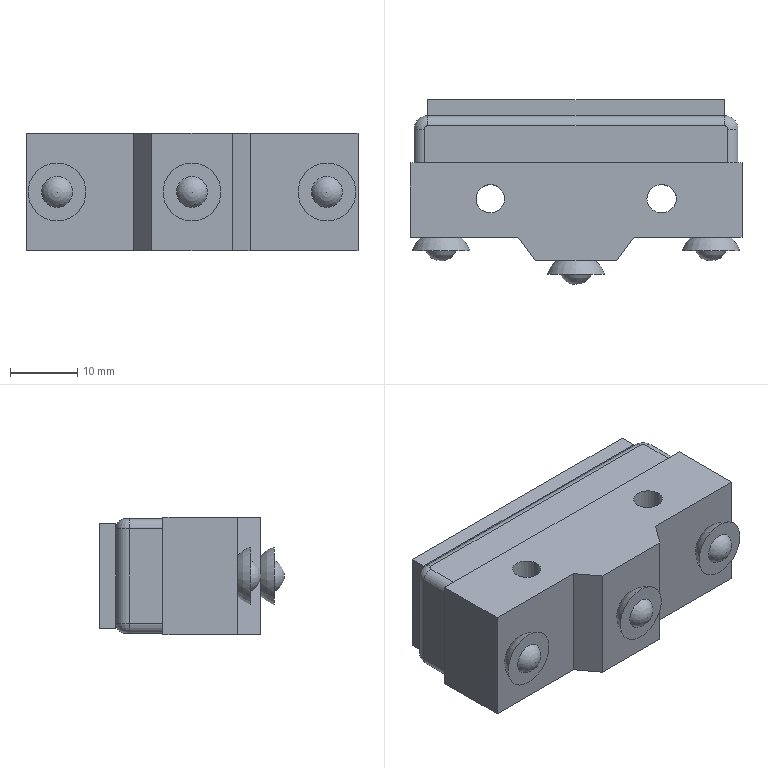Part | NX | features MFD10-WL40_1 2 | 1 solid | 44 faces | box 49.2 x 27.4 x 17.45 mm | volume 17430 mm3 | plane 24 | cylinder 9 | sphere 6 | torus 4 | spline 1 | commonest cylinder face diameters 3 x6 4 x2 4.2 x1
STEP:
#1=CARTESIAN_POINT('',(255.829,-488.15,79.));
#2=VERTEX_POINT('',#1);
#3=CARTESIAN_POINT('',(239.829,-488.15,79.));
#4=VERTEX_POINT('',#3);
#5=CARTESIAN_POINT('',(255.829,-488.15,79.));
#6=DIRECTION('',(-1.,0.,0.));
#7=VECTOR('',#6,1000.);
#8=LINE('',#5,#7);
#9=EDGE_CURVE('',#2,#4,#8,.T.);
#10=ORIENTED_EDGE('',*,*,#9,.F.);
#11=CARTESIAN_POINT('',(255.829,-488.15,96.45));
#12=VERTEX_POINT('',#11);
#13=CARTESIAN_POINT('',(255.829,-488.15,96.45));
#14=DIRECTION('',(0.,0.,-1.));
#15=VECTOR('',#14,1000.);
#16=LINE('',#13,#15);
#17=EDGE_CURVE('',#12,#2,#16,.T.);
#18=ORIENTED_EDGE('',*,*,#17,.F.);
#19=CARTESIAN_POINT('',(239.829,-488.15,96.45));
#20=VERTEX_POINT('',#19);
#21=CARTESIAN_POINT('',(255.829,-488.15,96.45));
#22=DIRECTION('',(-1.,0.,0.));
#23=VECTOR('',#22,1000.);
#24=LINE('',#21,#23);
#25=EDGE_CURVE('',#12,#20,#24,.T.);
#26=ORIENTED_EDGE('',*,*,#25,.T.);
#27=CARTESIAN_POINT('',(239.829,-488.15,96.45));
#28=DIRECTION('',(0.,0.,-1.));
#29=VECTOR('',#28,1000.);
#30=LINE('',#27,#29);
#31=EDGE_CURVE('',#20,#4,#30,.T.);
#32=ORIENTED_EDGE('',*,*,#31,.T.);
#33=EDGE_LOOP('',(#10,#18,#26,#32));
#34=FACE_BOUND('',#33,.T.);
#35=CARTESIAN_POINT('',(244.429,-488.15,90.725));
#36=VERTEX_POINT('',#35);
#37=CARTESIAN_POINT('',(244.429,-488.15,87.725));
#38=DIRECTION('',(0.,1.,0.));
#39=DIRECTION('',(0.,0.,1.));
#40=AXIS2_PLACEMENT_3D('',#37,#38,#39);
#41=CIRCLE('',#40,3.);
#42=EDGE_CURVE('',#36,#36,#41,.T.);
#43=ORIENTED_EDGE('',*,*,#42,.T.);
#44=EDGE_LOOP('',(#43));
#45=FACE_BOUND('',#44,.T.);
#46=CARTESIAN_POINT('',(255.829,-488.15,96.45));
#47=DIRECTION('',(0.,-1.,0.));
#48=DIRECTION('',(0.,0.,1.));
#49=AXIS2_PLACEMENT_3D('',#46,#47,#48);
#50=PLANE('',#49);
#51=ADVANCED_FACE('',(#34,#45),#50,.T.);
#52=CARTESIAN_POINT('',(289.029,-488.15,79.));
#53=VERTEX_POINT('',#52);
#54=CARTESIAN_POINT('',(273.029,-488.15,79.));
#55=VERTEX_POINT('',#54);
#56=CARTESIAN_POINT('',(289.029,-488.15,79.));
#57=DIRECTION('',(-1.,0.,0.));
#58=VECTOR('',#57,1000.);
#59=LINE('',#56,#58);
#60=EDGE_CURVE('',#53,#55,#59,.T.);
#61=ORIENTED_EDGE('',*,*,#60,.F.);
#62=CARTESIAN_POINT('',(289.029,-488.15,96.45));
#63=VERTEX_POINT('',#62);
#64=CARTESIAN_POINT('',(289.029,-488.15,96.45));
#65=DIRECTION('',(0.,0.,-1.));
#66=VECTOR('',#65,1000.);
#67=LINE('',#64,#66);
#68=EDGE_CURVE('',#63,#53,#67,.T.);
#69=ORIENTED_EDGE('',*,*,#68,.F.);
#70=CARTESIAN_POINT('',(273.029,-488.15,96.45));
#71=VERTEX_POINT('',#70);
#72=CARTESIAN_POINT('',(289.029,-488.15,96.45));
#73=DIRECTION('',(-1.,0.,0.));
#74=VECTOR('',#73,1000.);
#75=LINE('',#72,#74);
#76=EDGE_CURVE('',#63,#71,#75,.T.);
#77=ORIENTED_EDGE('',*,*,#76,.T.);
#78=CARTESIAN_POINT('',(273.029,-488.15,96.45));
#79=DIRECTION('',(0.,0.,-1.));
#80=VECTOR('',#79,1000.);
#81=LINE('',#78,#80);
#82=EDGE_CURVE('',#71,#55,#81,.T.);
#83=ORIENTED_EDGE('',*,*,#82,.T.);
#84=EDGE_LOOP('',(#61,#69,#77,#83));
#85=FACE_BOUND('',#84,.T.);
#86=CARTESIAN_POINT('',(284.429,-488.15,90.725));
#87=VERTEX_POINT('',#86);
#88=CARTESIAN_POINT('',(284.429,-488.15,87.725));
#89=DIRECTION('',(0.,-1.,0.));
#90=DIRECTION('',(0.,0.,1.));
#91=AXIS2_PLACEMENT_3D('',#88,#89,#90);
#92=CIRCLE('',#91,3.);
#93=EDGE_CURVE('',#87,#87,#92,.T.);
#94=ORIENTED_EDGE('',*,*,#93,.F.);
#95=EDGE_LOOP('',(#94));
#96=FACE_BOUND('',#95,.T.);
#97=CARTESIAN_POINT('',(289.029,-488.15,96.45));
#98=DIRECTION('',(0.,-1.,0.));
#99=DIRECTION('',(0.,0.,1.));
#100=AXIS2_PLACEMENT_3D('',#97,#98,#99);
#101=PLANE('',#100);
#102=ADVANCED_FACE('',(#85,#96),#101,.T.);
#103=CARTESIAN_POINT('',(270.429,-491.65,79.));
#104=VERTEX_POINT('',#103);
#105=CARTESIAN_POINT('',(258.429,-491.65,79.));
#106=VERTEX_POINT('',#105);
#107=CARTESIAN_POINT('',(270.429,-491.65,79.));
#108=DIRECTION('',(-1.,0.,0.));
#109=VECTOR('',#108,1000.);
#110=LINE('',#107,#109);
#111=EDGE_CURVE('',#104,#106,#110,.T.);
#112=ORIENTED_EDGE('',*,*,#111,.F.);
#113=CARTESIAN_POINT('',(270.429,-491.65,96.45));
#114=VERTEX_POINT('',#113);
#115=CARTESIAN_POINT('',(270.429,-491.65,96.45));
#116=DIRECTION('',(0.,0.,-1.));
#117=VECTOR('',#116,1000.);
#118=LINE('',#115,#117);
#119=EDGE_CURVE('',#114,#104,#118,.T.);
#120=ORIENTED_EDGE('',*,*,#119,.F.);
#121=CARTESIAN_POINT('',(258.429,-491.65,96.45));
#122=VERTEX_POINT('',#121);
#123=CARTESIAN_POINT('',(270.429,-491.65,96.45));
#124=DIRECTION('',(-1.,0.,0.));
#125=VECTOR('',#124,1000.);
#126=LINE('',#123,#125);
#127=EDGE_CURVE('',#114,#122,#126,.T.);
#128=ORIENTED_EDGE('',*,*,#127,.T.);
#129=CARTESIAN_POINT('',(258.429,-491.65,96.45));
#130=DIRECTION('',(0.,0.,-1.));
#131=VECTOR('',#130,1000.);
#132=LINE('',#129,#131);
#133=EDGE_CURVE('',#122,#106,#132,.T.);
#134=ORIENTED_EDGE('',*,*,#133,.T.);
#135=EDGE_LOOP('',(#112,#120,#128,#134));
#136=FACE_BOUND('',#135,.T.);
#137=CARTESIAN_POINT('',(264.429,-491.65,90.725));
#138=VERTEX_POINT('',#137);
#139=CARTESIAN_POINT('',(264.429,-491.65,87.725));
#140=DIRECTION('',(0.,-1.,0.));
#141=DIRECTION('',(0.,0.,1.));
#142=AXIS2_PLACEMENT_3D('',#139,#140,#141);
#143=CIRCLE('',#142,3.);
#144=EDGE_CURVE('',#138,#138,#143,.T.);
#145=ORIENTED_EDGE('',*,*,#144,.F.);
#146=EDGE_LOOP('',(#145));
#147=FACE_BOUND('',#146,.T.);
#148=CARTESIAN_POINT('',(270.429,-491.65,96.45));
#149=DIRECTION('',(0.,-1.,0.));
#150=DIRECTION('',(0.,0.,1.));
#151=AXIS2_PLACEMENT_3D('',#148,#149,#150);
#152=PLANE('',#151);
#153=ADVANCED_FACE('',(#136,#147),#152,.T.);
#154=CARTESIAN_POINT('',(273.029,-488.15,79.));
#155=DIRECTION('',(-0.5963,-0.8027,0.));
#156=VECTOR('',#155,1000.);
#157=LINE('',#154,#156);
#158=EDGE_CURVE('',#55,#104,#157,.T.);
#159=ORIENTED_EDGE('',*,*,#158,.F.);
#160=ORIENTED_EDGE('',*,*,#82,.F.);
#161=CARTESIAN_POINT('',(273.029,-488.15,96.45));
#162=DIRECTION('',(-0.5963,-0.8027,0.));
#163=VECTOR('',#162,1000.);
#164=LINE('',#161,#163);
#165=EDGE_CURVE('',#71,#114,#164,.T.);
#166=ORIENTED_EDGE('',*,*,#165,.T.);
#167=ORIENTED_EDGE('',*,*,#119,.T.);
#168=EDGE_LOOP('',(#159,#160,#166,#167));
#169=FACE_BOUND('',#168,.T.);
#170=CARTESIAN_POINT('',(273.029,-488.15,96.45));
#171=DIRECTION('',(0.8027,-0.5963,0.));
#172=DIRECTION('',(0.5963,0.8027,0.));
#173=AXIS2_PLACEMENT_3D('',#170,#171,#172);
#174=PLANE('',#173);
#175=ADVANCED_FACE('',(#169),#174,.T.);
#176=CARTESIAN_POINT('',(258.429,-491.65,79.));
#177=DIRECTION('',(-0.5963,0.8027,0.));
#178=VECTOR('',#177,1000.);
#179=LINE('',#176,#178);
#180=EDGE_CURVE('',#106,#2,#179,.T.);
#181=ORIENTED_EDGE('',*,*,#180,.F.);
#182=ORIENTED_EDGE('',*,*,#133,.F.);
#183=CARTESIAN_POINT('',(258.429,-491.65,96.45));
#184=DIRECTION('',(-0.5963,0.8027,0.));
#185=VECTOR('',#184,1000.);
#186=LINE('',#183,#185);
#187=EDGE_CURVE('',#122,#12,#186,.T.);
#188=ORIENTED_EDGE('',*,*,#187,.T.);
#189=ORIENTED_EDGE('',*,*,#17,.T.);
#190=EDGE_LOOP('',(#181,#182,#188,#189));
#191=FACE_BOUND('',#190,.T.);
#192=CARTESIAN_POINT('',(258.429,-491.65,96.45));
#193=DIRECTION('',(-0.8027,-0.5963,0.));
#194=DIRECTION('',(0.,0.,1.));
#195=AXIS2_PLACEMENT_3D('',#192,#193,#194);
#196=PLANE('',#195);
#197=ADVANCED_FACE('',(#191),#196,.T.);
#198=CARTESIAN_POINT('',(239.829,-477.15,79.));
#199=VERTEX_POINT('',#198);
#200=CARTESIAN_POINT('',(239.829,-488.15,79.));
#201=DIRECTION('',(0.,1.,0.));
#202=VECTOR('',#201,1000.);
#203=LINE('',#200,#202);
#204=EDGE_CURVE('',#4,#199,#203,.T.);
#205=ORIENTED_EDGE('',*,*,#204,.F.);
#206=ORIENTED_EDGE('',*,*,#31,.F.);
#207=CARTESIAN_POINT('',(239.829,-477.15,96.45));
#208=VERTEX_POINT('',#207);
#209=CARTESIAN_POINT('',(239.829,-488.15,96.45));
#210=DIRECTION('',(0.,1.,0.));
#211=VECTOR('',#210,1000.);
#212=LINE('',#209,#211);
#213=EDGE_CURVE('',#20,#208,#212,.T.);
#214=ORIENTED_EDGE('',*,*,#213,.T.);
#215=CARTESIAN_POINT('',(239.829,-477.15,96.45));
#216=DIRECTION('',(0.,0.,-1.));
#217=VECTOR('',#216,1000.);
#218=LINE('',#215,#217);
#219=EDGE_CURVE('',#208,#199,#218,.T.);
#220=ORIENTED_EDGE('',*,*,#219,.T.);
#221=EDGE_LOOP('',(#205,#206,#214,#220));
#222=FACE_BOUND('',#221,.T.);
#223=CARTESIAN_POINT('',(239.829,-488.15,96.45));
#224=DIRECTION('',(-1.,0.,0.));
#225=DIRECTION('',(0.,1.,0.));
#226=AXIS2_PLACEMENT_3D('',#223,#224,#225);
#227=PLANE('',#226);
#228=ADVANCED_FACE('',(#222),#227,.T.);
#229=CARTESIAN_POINT('',(289.029,-477.15,79.));
#230=VERTEX_POINT('',#229);
#231=CARTESIAN_POINT('',(239.829,-477.15,79.));
#232=DIRECTION('',(1.,0.,0.));
#233=VECTOR('',#232,1000.);
#234=LINE('',#231,#233);
#235=EDGE_CURVE('',#199,#230,#234,.T.);
#236=ORIENTED_EDGE('',*,*,#235,.F.);
#237=ORIENTED_EDGE('',*,*,#219,.F.);
#238=CARTESIAN_POINT('',(289.029,-477.15,96.45));
#239=VERTEX_POINT('',#238);
#240=CARTESIAN_POINT('',(239.829,-477.15,96.45));
#241=DIRECTION('',(1.,0.,0.));
#242=VECTOR('',#241,1000.);
#243=LINE('',#240,#242);
#244=EDGE_CURVE('',#208,#239,#243,.T.);
#245=ORIENTED_EDGE('',*,*,#244,.T.);
#246=CARTESIAN_POINT('',(289.029,-477.15,96.45));
#247=DIRECTION('',(0.,0.,-1.));
#248=VECTOR('',#247,1000.);
#249=LINE('',#246,#248);
#250=EDGE_CURVE('',#239,#230,#249,.T.);
#251=ORIENTED_EDGE('',*,*,#250,.T.);
#252=EDGE_LOOP('',(#236,#237,#245,#251));
#253=FACE_BOUND('',#252,.T.);
#254=CARTESIAN_POINT('',(241.929,-477.15,96.225));
#255=VERTEX_POINT('',#254);
#256=CARTESIAN_POINT('',(286.929,-477.15,96.225));
#257=VERTEX_POINT('',#256);
#258=CARTESIAN_POINT('',(240.429,-477.15,96.225));
#259=DIRECTION('',(1.,0.,0.));
#260=VECTOR('',#259,1000.);
#261=LINE('',#258,#260);
#262=EDGE_CURVE('',#255,#257,#261,.T.);
#263=ORIENTED_EDGE('',*,*,#262,.F.);
#264=CARTESIAN_POINT('',(240.429,-477.15,94.725));
#265=VERTEX_POINT('',#264);
#266=CARTESIAN_POINT('',(241.929,-477.15,94.725));
#267=DIRECTION('',(0.,-1.,0.));
#268=DIRECTION('',(0.,0.,-1.));
#269=AXIS2_PLACEMENT_3D('',#266,#267,#268);
#270=CIRCLE('',#269,1.5);
#271=EDGE_CURVE('',#255,#265,#270,.T.);
#272=ORIENTED_EDGE('',*,*,#271,.T.);
#273=CARTESIAN_POINT('',(240.429,-477.15,80.725));
#274=VERTEX_POINT('',#273);
#275=CARTESIAN_POINT('',(240.429,-477.15,96.225));
#276=DIRECTION('',(0.,0.,-1.));
#277=VECTOR('',#276,1000.);
#278=LINE('',#275,#277);
#279=EDGE_CURVE('',#265,#274,#278,.T.);
#280=ORIENTED_EDGE('',*,*,#279,.T.);
#281=CARTESIAN_POINT('',(241.929,-477.15,79.225));
#282=VERTEX_POINT('',#281);
#283=CARTESIAN_POINT('',(241.929,-477.15,80.725));
#284=DIRECTION('',(0.,-1.,0.));
#285=DIRECTION('',(0.,0.,-1.));
#286=AXIS2_PLACEMENT_3D('',#283,#284,#285);
#287=CIRCLE('',#286,1.5);
#288=EDGE_CURVE('',#274,#282,#287,.T.);
#289=ORIENTED_EDGE('',*,*,#288,.T.);
#290=CARTESIAN_POINT('',(286.929,-477.15,79.225));
#291=VERTEX_POINT('',#290);
#292=CARTESIAN_POINT('',(240.429,-477.15,79.225));
#293=DIRECTION('',(1.,0.,0.));
#294=VECTOR('',#293,1000.);
#295=LINE('',#292,#294);
#296=EDGE_CURVE('',#282,#291,#295,.T.);
#297=ORIENTED_EDGE('',*,*,#296,.T.);
#298=CARTESIAN_POINT('',(288.429,-477.15,80.725));
#299=VERTEX_POINT('',#298);
#300=CARTESIAN_POINT('',(286.929,-477.15,80.725));
#301=DIRECTION('',(0.,-1.,0.));
#302=DIRECTION('',(0.,0.,-1.));
#303=AXIS2_PLACEMENT_3D('',#300,#301,#302);
#304=CIRCLE('',#303,1.5);
#305=EDGE_CURVE('',#291,#299,#304,.T.);
#306=ORIENTED_EDGE('',*,*,#305,.T.);
#307=CARTESIAN_POINT('',(288.429,-477.15,94.725));
#308=VERTEX_POINT('',#307);
#309=CARTESIAN_POINT('',(288.429,-477.15,96.225));
#310=DIRECTION('',(0.,0.,-1.));
#311=VECTOR('',#310,1000.);
#312=LINE('',#309,#311);
#313=EDGE_CURVE('',#308,#299,#312,.T.);
#314=ORIENTED_EDGE('',*,*,#313,.F.);
#315=CARTESIAN_POINT('',(286.929,-477.15,94.725));
#316=DIRECTION('',(0.,-1.,0.));
#317=DIRECTION('',(0.,0.,-1.));
#318=AXIS2_PLACEMENT_3D('',#315,#316,#317);
#319=CIRCLE('',#318,1.5);
#320=EDGE_CURVE('',#308,#257,#319,.T.);
#321=ORIENTED_EDGE('',*,*,#320,.T.);
#322=EDGE_LOOP('',(#263,#272,#280,#289,#297,#306,#314,#321));
#323=FACE_BOUND('',#322,.T.);
#324=CARTESIAN_POINT('',(239.829,-477.15,96.45));
#325=DIRECTION('',(0.,1.,0.));
#326=DIRECTION('',(-1.,0.,0.));
#327=AXIS2_PLACEMENT_3D('',#324,#325,#326);
#328=PLANE('',#327);
#329=ADVANCED_FACE('',(#253,#323),#328,.T.);
#330=CARTESIAN_POINT('',(289.029,-477.15,79.));
#331=DIRECTION('',(0.,-1.,0.));
#332=VECTOR('',#331,1000.);
#333=LINE('',#330,#332);
#334=EDGE_CURVE('',#230,#53,#333,.T.);
#335=ORIENTED_EDGE('',*,*,#334,.F.);
#336=ORIENTED_EDGE('',*,*,#250,.F.);
#337=CARTESIAN_POINT('',(289.029,-477.15,96.45));
#338=DIRECTION('',(0.,-1.,0.));
#339=VECTOR('',#338,1000.);
#340=LINE('',#337,#339);
#341=EDGE_CURVE('',#239,#63,#340,.T.);
#342=ORIENTED_EDGE('',*,*,#341,.T.);
#343=ORIENTED_EDGE('',*,*,#68,.T.);
#344=EDGE_LOOP('',(#335,#336,#342,#343));
#345=FACE_BOUND('',#344,.T.);
#346=CARTESIAN_POINT('',(289.029,-477.15,96.45));
#347=DIRECTION('',(1.,0.,0.));
#348=DIRECTION('',(0.,0.,-1.));
#349=AXIS2_PLACEMENT_3D('',#346,#347,#348);
#350=PLANE('',#349);
#351=ADVANCED_FACE('',(#345),#350,.T.);
#352=CARTESIAN_POINT('',(274.949,-482.45,96.45));
#353=VERTEX_POINT('',#352);
#354=CARTESIAN_POINT('',(277.129,-482.45,96.45));
#355=DIRECTION('',(0.,0.,-1.));
#356=DIRECTION('',(-1.,0.,0.));
#357=AXIS2_PLACEMENT_3D('',#354,#355,#356);
#358=ELLIPSE('',#357,2.18,2.1);
#359=EDGE_CURVE('',#353,#353,#358,.T.);
#360=ORIENTED_EDGE('',*,*,#359,.F.);
#361=EDGE_LOOP('',(#360));
#362=FACE_BOUND('',#361,.T.);
#363=CARTESIAN_POINT('',(274.949,-482.45,79.));
#364=VERTEX_POINT('',#363);
#365=CARTESIAN_POINT('',(277.129,-482.45,79.));
#366=DIRECTION('',(0.,0.,-1.));
#367=DIRECTION('',(-1.,0.,0.));
#368=AXIS2_PLACEMENT_3D('',#365,#366,#367);
#369=ELLIPSE('',#368,2.18,2.1);
#370=EDGE_CURVE('',#364,#364,#369,.T.);
#371=ORIENTED_EDGE('',*,*,#370,.T.);
#372=EDGE_LOOP('',(#371));
#373=FACE_BOUND('',#372,.T.);
#374=CARTESIAN_POINT('',(275.42,-484.096,96.45));
#375=CARTESIAN_POINT('',(275.42,-484.096,79.));
#376=CARTESIAN_POINT('',(274.713,-482.45,96.45));
#377=CARTESIAN_POINT('',(274.713,-482.45,79.));
#378=CARTESIAN_POINT('',(275.42,-480.804,96.45));
#379=CARTESIAN_POINT('',(275.42,-480.804,79.));
#380=CARTESIAN_POINT('',(277.129,-480.123,96.45));
#381=CARTESIAN_POINT('',(277.129,-480.123,79.));
#382=CARTESIAN_POINT('',(278.837,-480.804,96.45));
#383=CARTESIAN_POINT('',(278.837,-480.804,79.));
#384=CARTESIAN_POINT('',(279.544,-482.45,96.45));
#385=CARTESIAN_POINT('',(279.544,-482.45,79.));
#386=CARTESIAN_POINT('',(278.837,-484.096,96.45));
#387=CARTESIAN_POINT('',(278.837,-484.096,79.));
#388=CARTESIAN_POINT('',(277.129,-484.777,96.45));
#389=CARTESIAN_POINT('',(277.129,-484.777,79.));
#390=CARTESIAN_POINT('',(275.42,-484.096,96.45));
#391=CARTESIAN_POINT('',(275.42,-484.096,79.));
#392=CARTESIAN_POINT('',(274.713,-482.45,96.45));
#393=CARTESIAN_POINT('',(274.713,-482.45,79.));
#394=CARTESIAN_POINT('',(275.42,-480.804,96.45));
#395=CARTESIAN_POINT('',(275.42,-480.804,79.));
#396=B_SPLINE_SURFACE_WITH_KNOTS('',3,1,((#374,#375),(#376,#377),(#378,#379),(#380,#381),(#382,#383),(#384,#385),(#386,#387),(#388,#389),(#390,#391),(#392,#393),(#394,#395)),.SURF_OF_LINEAR_EXTRUSION.,.T.,.F.,.F.,(1,1,1,1,1,1,1,1,1,1,1,1,1,1,1),(2,2),(-2.356,-1.571,-0.7854,0.,0.7854,1.571,2.356,3.142,3.927,4.712,5.498,6.283,7.069,7.854,8.639),(0.,1.),.UNSPECIFIED.);
#397=ADVANCED_FACE('',(#362,#373),#396,.F.);
#398=CARTESIAN_POINT('',(249.629,-482.45,96.45));
#399=VERTEX_POINT('',#398);
#400=CARTESIAN_POINT('',(251.729,-482.45,96.45));
#401=DIRECTION('',(0.,0.,-1.));
#402=DIRECTION('',(-1.,0.,0.));
#403=AXIS2_PLACEMENT_3D('',#400,#401,#402);
#404=CIRCLE('',#403,2.1);
#405=EDGE_CURVE('',#399,#399,#404,.T.);
#406=ORIENTED_EDGE('',*,*,#405,.F.);
#407=EDGE_LOOP('',(#406));
#408=FACE_BOUND('',#407,.T.);
#409=CARTESIAN_POINT('',(249.629,-482.45,79.));
#410=VERTEX_POINT('',#409);
#411=CARTESIAN_POINT('',(251.729,-482.45,79.));
#412=DIRECTION('',(0.,0.,-1.));
#413=DIRECTION('',(-1.,0.,0.));
#414=AXIS2_PLACEMENT_3D('',#411,#412,#413);
#415=CIRCLE('',#414,2.1);
#416=EDGE_CURVE('',#410,#410,#415,.T.);
#417=ORIENTED_EDGE('',*,*,#416,.T.);
#418=EDGE_LOOP('',(#417));
#419=FACE_BOUND('',#418,.T.);
#420=CARTESIAN_POINT('',(251.729,-482.45,96.45));
#421=DIRECTION('',(0.,0.,1.));
#422=DIRECTION('',(-1.,0.,0.));
#423=AXIS2_PLACEMENT_3D('',#420,#421,#422);
#424=CYLINDRICAL_SURFACE('',#423,2.1);
#425=ADVANCED_FACE('',(#408,#419),#424,.F.);
#426=ORIENTED_EDGE('',*,*,#165,.F.);
#427=ORIENTED_EDGE('',*,*,#76,.F.);
#428=ORIENTED_EDGE('',*,*,#341,.F.);
#429=ORIENTED_EDGE('',*,*,#244,.F.);
#430=ORIENTED_EDGE('',*,*,#213,.F.);
#431=ORIENTED_EDGE('',*,*,#25,.F.);
#432=ORIENTED_EDGE('',*,*,#187,.F.);
#433=ORIENTED_EDGE('',*,*,#127,.F.);
#434=EDGE_LOOP('',(#426,#427,#428,#429,#430,#431,#432,#433));
#435=FACE_BOUND('',#434,.T.);
#436=ORIENTED_EDGE('',*,*,#359,.T.);
#437=EDGE_LOOP('',(#436));
#438=FACE_BOUND('',#437,.T.);
#439=ORIENTED_EDGE('',*,*,#405,.T.);
#440=EDGE_LOOP('',(#439));
#441=FACE_BOUND('',#440,.T.);
#442=CARTESIAN_POINT('',(277.129,-482.45,96.45));
#443=DIRECTION('',(0.,0.,-1.));
#444=DIRECTION('',(-1.,0.,0.));
#445=AXIS2_PLACEMENT_3D('',#442,#443,#444);
#446=PLANE('',#445);
#447=ADVANCED_FACE('',(#435,#438,#441),#446,.F.);
#448=ORIENTED_EDGE('',*,*,#158,.T.);
#449=ORIENTED_EDGE('',*,*,#111,.T.);
#450=ORIENTED_EDGE('',*,*,#180,.T.);
#451=ORIENTED_EDGE('',*,*,#9,.T.);
#452=ORIENTED_EDGE('',*,*,#204,.T.);
#453=ORIENTED_EDGE('',*,*,#235,.T.);
#454=ORIENTED_EDGE('',*,*,#334,.T.);
#455=ORIENTED_EDGE('',*,*,#60,.T.);
#456=EDGE_LOOP('',(#448,#449,#450,#451,#452,#453,#454,#455));
#457=FACE_BOUND('',#456,.T.);
#458=ORIENTED_EDGE('',*,*,#370,.F.);
#459=EDGE_LOOP('',(#458));
#460=FACE_BOUND('',#459,.T.);
#461=ORIENTED_EDGE('',*,*,#416,.F.);
#462=EDGE_LOOP('',(#461));
#463=FACE_BOUND('',#462,.T.);
#464=CARTESIAN_POINT('',(277.129,-482.45,79.));
#465=DIRECTION('',(0.,0.,-1.));
#466=DIRECTION('',(-1.,0.,0.));
#467=AXIS2_PLACEMENT_3D('',#464,#465,#466);
#468=PLANE('',#467);
#469=ADVANCED_FACE('',(#457,#460,#463),#468,.T.);
#470=CARTESIAN_POINT('',(240.429,-472.15,94.725));
#471=VERTEX_POINT('',#470);
#472=CARTESIAN_POINT('',(240.429,-472.15,80.725));
#473=VERTEX_POINT('',#472);
#474=CARTESIAN_POINT('',(240.429,-472.15,96.225));
#475=DIRECTION('',(0.,0.,-1.));
#476=VECTOR('',#475,1000.);
#477=LINE('',#474,#476);
#478=EDGE_CURVE('',#471,#473,#477,.T.);
#479=ORIENTED_EDGE('',*,*,#478,.T.);
#480=CARTESIAN_POINT('',(240.429,-470.15,80.725));
#481=DIRECTION('',(0.,-1.,0.));
#482=VECTOR('',#481,1000.);
#483=LINE('',#480,#482);
#484=EDGE_CURVE('',#473,#274,#483,.T.);
#485=ORIENTED_EDGE('',*,*,#484,.T.);
#486=ORIENTED_EDGE('',*,*,#279,.F.);
#487=CARTESIAN_POINT('',(240.429,-472.15,94.725));
#488=DIRECTION('',(0.,1.,0.));
#489=VECTOR('',#488,1000.);
#490=LINE('',#487,#489);
#491=EDGE_CURVE('',#265,#471,#490,.T.);
#492=ORIENTED_EDGE('',*,*,#491,.T.);
#493=EDGE_LOOP('',(#479,#485,#486,#492));
#494=FACE_BOUND('',#493,.T.);
#495=CARTESIAN_POINT('',(240.429,-470.15,96.225));
#496=DIRECTION('',(1.,0.,0.));
#497=DIRECTION('',(0.,0.,-1.));
#498=AXIS2_PLACEMENT_3D('',#495,#496,#497);
#499=PLANE('',#498);
#500=ADVANCED_FACE('',(#494),#499,.F.);
#501=ORIENTED_EDGE('',*,*,#313,.T.);
#502=CARTESIAN_POINT('',(288.429,-472.15,80.725));
#503=VERTEX_POINT('',#502);
#504=CARTESIAN_POINT('',(288.429,-477.15,80.725));
#505=DIRECTION('',(0.,1.,0.));
#506=VECTOR('',#505,1000.);
#507=LINE('',#504,#506);
#508=EDGE_CURVE('',#299,#503,#507,.T.);
#509=ORIENTED_EDGE('',*,*,#508,.T.);
#510=CARTESIAN_POINT('',(288.429,-472.15,94.725));
#511=VERTEX_POINT('',#510);
#512=CARTESIAN_POINT('',(288.429,-472.15,96.225));
#513=DIRECTION('',(0.,0.,1.));
#514=VECTOR('',#513,1000.);
#515=LINE('',#512,#514);
#516=EDGE_CURVE('',#503,#511,#515,.T.);
#517=ORIENTED_EDGE('',*,*,#516,.T.);
#518=CARTESIAN_POINT('',(288.429,-477.15,94.725));
#519=DIRECTION('',(0.,-1.,0.));
#520=VECTOR('',#519,1000.);
#521=LINE('',#518,#520);
#522=EDGE_CURVE('',#511,#308,#521,.T.);
#523=ORIENTED_EDGE('',*,*,#522,.T.);
#524=EDGE_LOOP('',(#501,#509,#517,#523));
#525=FACE_BOUND('',#524,.T.);
#526=CARTESIAN_POINT('',(288.429,-477.15,96.225));
#527=DIRECTION('',(-1.,0.,0.));
#528=DIRECTION('',(0.,1.,0.));
#529=AXIS2_PLACEMENT_3D('',#526,#527,#528);
#530=PLANE('',#529);
#531=ADVANCED_FACE('',(#525),#530,.F.);
#532=ORIENTED_EDGE('',*,*,#262,.T.);
#533=CARTESIAN_POINT('',(286.929,-472.15,96.225));
#534=VERTEX_POINT('',#533);
#535=CARTESIAN_POINT('',(286.929,-472.15,96.225));
#536=DIRECTION('',(0.,1.,0.));
#537=VECTOR('',#536,1000.);
#538=LINE('',#535,#537);
#539=EDGE_CURVE('',#257,#534,#538,.T.);
#540=ORIENTED_EDGE('',*,*,#539,.T.);
#541=CARTESIAN_POINT('',(286.429,-471.65,96.225));
#542=VERTEX_POINT('',#541);
#543=CARTESIAN_POINT('',(286.429,-472.15,96.225));
#544=DIRECTION('',(0.,0.,1.));
#545=DIRECTION('',(1.,0.,0.));
#546=AXIS2_PLACEMENT_3D('',#543,#544,#545);
#547=CIRCLE('',#546,0.5);
#548=EDGE_CURVE('',#534,#542,#547,.T.);
#549=ORIENTED_EDGE('',*,*,#548,.T.);
#550=CARTESIAN_POINT('',(242.429,-471.65,96.225));
#551=VERTEX_POINT('',#550);
#552=CARTESIAN_POINT('',(242.429,-471.65,96.225));
#553=DIRECTION('',(-1.,0.,0.));
#554=VECTOR('',#553,1000.);
#555=LINE('',#552,#554);
#556=EDGE_CURVE('',#542,#551,#555,.T.);
#557=ORIENTED_EDGE('',*,*,#556,.T.);
#558=CARTESIAN_POINT('',(241.929,-472.15,96.225));
#559=VERTEX_POINT('',#558);
#560=CARTESIAN_POINT('',(242.429,-472.15,96.225));
#561=DIRECTION('',(0.,0.,1.));
#562=DIRECTION('',(1.,0.,0.));
#563=AXIS2_PLACEMENT_3D('',#560,#561,#562);
#564=CIRCLE('',#563,0.5);
#565=EDGE_CURVE('',#551,#559,#564,.T.);
#566=ORIENTED_EDGE('',*,*,#565,.T.);
#567=CARTESIAN_POINT('',(241.929,-477.15,96.225));
#568=DIRECTION('',(0.,-1.,0.));
#569=VECTOR('',#568,1000.);
#570=LINE('',#567,#569);
#571=EDGE_CURVE('',#559,#255,#570,.T.);
#572=ORIENTED_EDGE('',*,*,#571,.T.);
#573=EDGE_LOOP('',(#532,#540,#549,#557,#566,#572));
#574=FACE_BOUND('',#573,.T.);
#575=CARTESIAN_POINT('',(240.429,-470.15,96.225));
#576=DIRECTION('',(0.,0.,1.));
#577=DIRECTION('',(0.,-1.,0.));
#578=AXIS2_PLACEMENT_3D('',#575,#576,#577);
#579=PLANE('',#578);
#580=ADVANCED_FACE('',(#574),#579,.T.);
#581=CARTESIAN_POINT('',(286.429,-471.65,79.225));
#582=VERTEX_POINT('',#581);
#583=CARTESIAN_POINT('',(286.929,-472.15,79.225));
#584=VERTEX_POINT('',#583);
#585=CARTESIAN_POINT('',(286.429,-472.15,79.225));
#586=DIRECTION('',(0.,0.,-1.));
#587=DIRECTION('',(1.,0.,0.));
#588=AXIS2_PLACEMENT_3D('',#585,#586,#587);
#589=CIRCLE('',#588,0.5);
#590=EDGE_CURVE('',#582,#584,#589,.T.);
#591=ORIENTED_EDGE('',*,*,#590,.T.);
#592=CARTESIAN_POINT('',(286.929,-470.15,79.225));
#593=DIRECTION('',(0.,-1.,0.));
#594=VECTOR('',#593,1000.);
#595=LINE('',#592,#594);
#596=EDGE_CURVE('',#584,#291,#595,.T.);
#597=ORIENTED_EDGE('',*,*,#596,.T.);
#598=ORIENTED_EDGE('',*,*,#296,.F.);
#599=CARTESIAN_POINT('',(241.929,-472.15,79.225));
#600=VERTEX_POINT('',#599);
#601=CARTESIAN_POINT('',(241.929,-470.15,79.225));
#602=DIRECTION('',(0.,1.,0.));
#603=VECTOR('',#602,1000.);
#604=LINE('',#601,#603);
#605=EDGE_CURVE('',#282,#600,#604,.T.);
#606=ORIENTED_EDGE('',*,*,#605,.T.);
#607=CARTESIAN_POINT('',(242.429,-471.65,79.225));
#608=VERTEX_POINT('',#607);
#609=CARTESIAN_POINT('',(242.429,-472.15,79.225));
#610=DIRECTION('',(0.,0.,-1.));
#611=DIRECTION('',(1.,0.,0.));
#612=AXIS2_PLACEMENT_3D('',#609,#610,#611);
#613=CIRCLE('',#612,0.5);
#614=EDGE_CURVE('',#600,#608,#613,.T.);
#615=ORIENTED_EDGE('',*,*,#614,.T.);
#616=CARTESIAN_POINT('',(240.429,-471.65,79.225));
#617=DIRECTION('',(1.,0.,0.));
#618=VECTOR('',#617,1000.);
#619=LINE('',#616,#618);
#620=EDGE_CURVE('',#608,#582,#619,.T.);
#621=ORIENTED_EDGE('',*,*,#620,.T.);
#622=EDGE_LOOP('',(#591,#597,#598,#606,#615,#621));
#623=FACE_BOUND('',#622,.T.);
#624=CARTESIAN_POINT('',(240.429,-470.15,79.225));
#625=DIRECTION('',(0.,0.,1.));
#626=DIRECTION('',(0.,-1.,0.));
#627=AXIS2_PLACEMENT_3D('',#624,#625,#626);
#628=PLANE('',#627);
#629=ADVANCED_FACE('',(#623),#628,.F.);
#630=CARTESIAN_POINT('',(242.429,-470.15,80.725));
#631=VERTEX_POINT('',#630);
#632=CARTESIAN_POINT('',(242.429,-470.15,94.725));
#633=VERTEX_POINT('',#632);
#634=CARTESIAN_POINT('',(242.429,-470.15,96.225));
#635=DIRECTION('',(0.,0.,1.));
#636=VECTOR('',#635,1000.);
#637=LINE('',#634,#636);
#638=EDGE_CURVE('',#631,#633,#637,.T.);
#639=ORIENTED_EDGE('',*,*,#638,.F.);
#640=CARTESIAN_POINT('',(242.429,-472.15,80.725));
#641=DIRECTION('',(0.,0.,1.));
#642=DIRECTION('',(1.,0.,0.));
#643=AXIS2_PLACEMENT_3D('',#640,#641,#642);
#644=CIRCLE('',#643,2.);
#645=EDGE_CURVE('',#631,#473,#644,.T.);
#646=ORIENTED_EDGE('',*,*,#645,.T.);
#647=ORIENTED_EDGE('',*,*,#478,.F.);
#648=CARTESIAN_POINT('',(242.429,-472.15,94.725));
#649=DIRECTION('',(0.,0.,-1.));
#650=DIRECTION('',(1.,0.,0.));
#651=AXIS2_PLACEMENT_3D('',#648,#649,#650);
#652=CIRCLE('',#651,2.);
#653=EDGE_CURVE('',#471,#633,#652,.T.);
#654=ORIENTED_EDGE('',*,*,#653,.T.);
#655=EDGE_LOOP('',(#639,#646,#647,#654));
#656=FACE_BOUND('',#655,.T.);
#657=CARTESIAN_POINT('',(242.429,-472.15,96.225));
#658=DIRECTION('',(0.,0.,1.));
#659=DIRECTION('',(-1.,0.,0.));
#660=AXIS2_PLACEMENT_3D('',#657,#658,#659);
#661=CYLINDRICAL_SURFACE('',#660,2.);
#662=ADVANCED_FACE('',(#656),#661,.T.);
#663=ORIENTED_EDGE('',*,*,#516,.F.);
#664=CARTESIAN_POINT('',(286.429,-470.15,80.725));
#665=VERTEX_POINT('',#664);
#666=CARTESIAN_POINT('',(286.429,-472.15,80.725));
#667=DIRECTION('',(0.,0.,1.));
#668=DIRECTION('',(1.,0.,0.));
#669=AXIS2_PLACEMENT_3D('',#666,#667,#668);
#670=CIRCLE('',#669,2.);
#671=EDGE_CURVE('',#503,#665,#670,.T.);
#672=ORIENTED_EDGE('',*,*,#671,.T.);
#673=CARTESIAN_POINT('',(286.429,-470.15,94.725));
#674=VERTEX_POINT('',#673);
#675=CARTESIAN_POINT('',(286.429,-470.15,96.225));
#676=DIRECTION('',(0.,0.,-1.));
#677=VECTOR('',#676,1000.);
#678=LINE('',#675,#677);
#679=EDGE_CURVE('',#674,#665,#678,.T.);
#680=ORIENTED_EDGE('',*,*,#679,.F.);
#681=CARTESIAN_POINT('',(286.429,-472.15,94.725));
#682=DIRECTION('',(0.,0.,-1.));
#683=DIRECTION('',(1.,0.,0.));
#684=AXIS2_PLACEMENT_3D('',#681,#682,#683);
#685=CIRCLE('',#684,2.);
#686=EDGE_CURVE('',#674,#511,#685,.T.);
#687=ORIENTED_EDGE('',*,*,#686,.T.);
#688=EDGE_LOOP('',(#663,#672,#680,#687));
#689=FACE_BOUND('',#688,.T.);
#690=CARTESIAN_POINT('',(286.429,-472.15,96.225));
#691=DIRECTION('',(0.,0.,1.));
#692=DIRECTION('',(-1.,0.,0.));
#693=AXIS2_PLACEMENT_3D('',#690,#691,#692);
#694=CYLINDRICAL_SURFACE('',#693,2.);
#695=ADVANCED_FACE('',(#689),#694,.T.);
#696=ORIENTED_EDGE('',*,*,#288,.F.);
#697=ORIENTED_EDGE('',*,*,#484,.F.);
#698=CARTESIAN_POINT('',(241.929,-472.15,80.725));
#699=DIRECTION('',(0.,1.,0.));
#700=DIRECTION('',(0.,0.,-1.));
#701=AXIS2_PLACEMENT_3D('',#698,#699,#700);
#702=CIRCLE('',#701,1.5);
#703=EDGE_CURVE('',#600,#473,#702,.T.);
#704=ORIENTED_EDGE('',*,*,#703,.F.);
#705=ORIENTED_EDGE('',*,*,#605,.F.);
#706=EDGE_LOOP('',(#696,#697,#704,#705));
#707=FACE_BOUND('',#706,.T.);
#708=CARTESIAN_POINT('',(241.929,-470.15,80.725));
#709=DIRECTION('',(0.,1.,0.));
#710=DIRECTION('',(0.,0.,1.));
#711=AXIS2_PLACEMENT_3D('',#708,#709,#710);
#712=CYLINDRICAL_SURFACE('',#711,1.5);
#713=ADVANCED_FACE('',(#707),#712,.T.);
#714=ORIENTED_EDGE('',*,*,#703,.T.);
#715=ORIENTED_EDGE('',*,*,#645,.F.);
#716=CARTESIAN_POINT('',(242.429,-471.65,80.725));
#717=DIRECTION('',(1.,0.,0.));
#718=DIRECTION('',(0.,0.,-1.));
#719=AXIS2_PLACEMENT_3D('',#716,#717,#718);
#720=CIRCLE('',#719,1.5);
#721=EDGE_CURVE('',#608,#631,#720,.T.);
#722=ORIENTED_EDGE('',*,*,#721,.F.);
#723=ORIENTED_EDGE('',*,*,#614,.F.);
#724=EDGE_LOOP('',(#714,#715,#722,#723));
#725=FACE_BOUND('',#724,.T.);
#726=CARTESIAN_POINT('',(242.429,-472.15,80.725));
#727=DIRECTION('',(0.,0.,1.));
#728=DIRECTION('',(0.,-1.,0.));
#729=AXIS2_PLACEMENT_3D('',#726,#727,#728);
#730=DEGENERATE_TOROIDAL_SURFACE('',#729,0.5,1.5,.T.);
#731=ADVANCED_FACE('',(#725),#730,.T.);
#732=ORIENTED_EDGE('',*,*,#721,.T.);
#733=CARTESIAN_POINT('',(288.429,-470.15,80.725));
#734=DIRECTION('',(-1.,0.,0.));
#735=VECTOR('',#734,1000.);
#736=LINE('',#733,#735);
#737=EDGE_CURVE('',#665,#631,#736,.T.);
#738=ORIENTED_EDGE('',*,*,#737,.F.);
#739=CARTESIAN_POINT('',(286.429,-471.65,80.725));
#740=DIRECTION('',(1.,0.,0.));
#741=DIRECTION('',(0.,0.,-1.));
#742=AXIS2_PLACEMENT_3D('',#739,#740,#741);
#743=CIRCLE('',#742,1.5);
#744=EDGE_CURVE('',#582,#665,#743,.T.);
#745=ORIENTED_EDGE('',*,*,#744,.F.);
#746=ORIENTED_EDGE('',*,*,#620,.F.);
#747=EDGE_LOOP('',(#732,#738,#745,#746));
#748=FACE_BOUND('',#747,.T.);
#749=CARTESIAN_POINT('',(288.429,-471.65,80.725));
#750=DIRECTION('',(1.,0.,0.));
#751=DIRECTION('',(0.,0.,1.));
#752=AXIS2_PLACEMENT_3D('',#749,#750,#751);
#753=CYLINDRICAL_SURFACE('',#752,1.5);
#754=ADVANCED_FACE('',(#748),#753,.T.);
#755=ORIENTED_EDGE('',*,*,#744,.T.);
#756=ORIENTED_EDGE('',*,*,#671,.F.);
#757=CARTESIAN_POINT('',(286.929,-472.15,80.725));
#758=DIRECTION('',(0.,-1.,0.));
#759=DIRECTION('',(0.,0.,1.));
#760=AXIS2_PLACEMENT_3D('',#757,#758,#759);
#761=CIRCLE('',#760,1.5);
#762=EDGE_CURVE('',#584,#503,#761,.T.);
#763=ORIENTED_EDGE('',*,*,#762,.F.);
#764=ORIENTED_EDGE('',*,*,#590,.F.);
#765=EDGE_LOOP('',(#755,#756,#763,#764));
#766=FACE_BOUND('',#765,.T.);
#767=CARTESIAN_POINT('',(286.429,-472.15,80.725));
#768=DIRECTION('',(0.,0.,1.));
#769=DIRECTION('',(1.,0.,0.));
#770=AXIS2_PLACEMENT_3D('',#767,#768,#769);
#771=DEGENERATE_TOROIDAL_SURFACE('',#770,0.5,1.5,.T.);
#772=ADVANCED_FACE('',(#766),#771,.T.);
#773=ORIENTED_EDGE('',*,*,#305,.F.);
#774=ORIENTED_EDGE('',*,*,#596,.F.);
#775=ORIENTED_EDGE('',*,*,#762,.T.);
#776=ORIENTED_EDGE('',*,*,#508,.F.);
#777=EDGE_LOOP('',(#773,#774,#775,#776));
#778=FACE_BOUND('',#777,.T.);
#779=CARTESIAN_POINT('',(286.929,-477.15,80.725));
#780=DIRECTION('',(0.,-1.,0.));
#781=DIRECTION('',(0.,0.,-1.));
#782=AXIS2_PLACEMENT_3D('',#779,#780,#781);
#783=CYLINDRICAL_SURFACE('',#782,1.5);
#784=ADVANCED_FACE('',(#778),#783,.T.);
#785=ORIENTED_EDGE('',*,*,#271,.F.);
#786=ORIENTED_EDGE('',*,*,#571,.F.);
#787=CARTESIAN_POINT('',(241.929,-472.15,94.725));
#788=DIRECTION('',(0.,1.,0.));
#789=DIRECTION('',(0.,0.,-1.));
#790=AXIS2_PLACEMENT_3D('',#787,#788,#789);
#791=CIRCLE('',#790,1.5);
#792=EDGE_CURVE('',#471,#559,#791,.T.);
#793=ORIENTED_EDGE('',*,*,#792,.F.);
#794=ORIENTED_EDGE('',*,*,#491,.F.);
#795=EDGE_LOOP('',(#785,#786,#793,#794));
#796=FACE_BOUND('',#795,.T.);
#797=CARTESIAN_POINT('',(241.929,-470.15,94.725));
#798=DIRECTION('',(0.,-1.,0.));
#799=DIRECTION('',(0.,0.,-1.));
#800=AXIS2_PLACEMENT_3D('',#797,#798,#799);
#801=CYLINDRICAL_SURFACE('',#800,1.5);
#802=ADVANCED_FACE('',(#796),#801,.T.);
#803=ORIENTED_EDGE('',*,*,#792,.T.);
#804=ORIENTED_EDGE('',*,*,#565,.F.);
#805=CARTESIAN_POINT('',(242.429,-471.65,94.725));
#806=DIRECTION('',(1.,0.,0.));
#807=DIRECTION('',(0.,0.,-1.));
#808=AXIS2_PLACEMENT_3D('',#805,#806,#807);
#809=CIRCLE('',#808,1.5);
#810=EDGE_CURVE('',#633,#551,#809,.T.);
#811=ORIENTED_EDGE('',*,*,#810,.F.);
#812=ORIENTED_EDGE('',*,*,#653,.F.);
#813=EDGE_LOOP('',(#803,#804,#811,#812));
#814=FACE_BOUND('',#813,.T.);
#815=CARTESIAN_POINT('',(242.429,-472.15,94.725));
#816=DIRECTION('',(0.,0.,1.));
#817=DIRECTION('',(1.,0.,0.));
#818=AXIS2_PLACEMENT_3D('',#815,#816,#817);
#819=DEGENERATE_TOROIDAL_SURFACE('',#818,0.5,1.5,.T.);
#820=ADVANCED_FACE('',(#814),#819,.T.);
#821=ORIENTED_EDGE('',*,*,#810,.T.);
#822=ORIENTED_EDGE('',*,*,#556,.F.);
#823=CARTESIAN_POINT('',(286.429,-471.65,94.725));
#824=DIRECTION('',(1.,0.,0.));
#825=DIRECTION('',(0.,0.,-1.));
#826=AXIS2_PLACEMENT_3D('',#823,#824,#825);
#827=CIRCLE('',#826,1.5);
#828=EDGE_CURVE('',#674,#542,#827,.T.);
#829=ORIENTED_EDGE('',*,*,#828,.F.);
#830=CARTESIAN_POINT('',(286.429,-470.15,94.725));
#831=DIRECTION('',(1.,0.,0.));
#832=VECTOR('',#831,1000.);
#833=LINE('',#830,#832);
#834=EDGE_CURVE('',#633,#674,#833,.T.);
#835=ORIENTED_EDGE('',*,*,#834,.F.);
#836=EDGE_LOOP('',(#821,#822,#829,#835));
#837=FACE_BOUND('',#836,.T.);
#838=CARTESIAN_POINT('',(240.429,-471.65,94.725));
#839=DIRECTION('',(-1.,0.,0.));
#840=DIRECTION('',(0.,0.,-1.));
#841=AXIS2_PLACEMENT_3D('',#838,#839,#840);
#842=CYLINDRICAL_SURFACE('',#841,1.5);
#843=ADVANCED_FACE('',(#837),#842,.T.);
#844=ORIENTED_EDGE('',*,*,#828,.T.);
#845=ORIENTED_EDGE('',*,*,#548,.F.);
#846=CARTESIAN_POINT('',(286.929,-472.15,94.725));
#847=DIRECTION('',(0.,-1.,0.));
#848=DIRECTION('',(0.,0.,1.));
#849=AXIS2_PLACEMENT_3D('',#846,#847,#848);
#850=CIRCLE('',#849,1.5);
#851=EDGE_CURVE('',#511,#534,#850,.T.);
#852=ORIENTED_EDGE('',*,*,#851,.F.);
#853=ORIENTED_EDGE('',*,*,#686,.F.);
#854=EDGE_LOOP('',(#844,#845,#852,#853));
#855=FACE_BOUND('',#854,.T.);
#856=CARTESIAN_POINT('',(286.429,-472.15,94.725));
#857=DIRECTION('',(0.,0.,1.));
#858=DIRECTION('',(1.,0.,0.));
#859=AXIS2_PLACEMENT_3D('',#856,#857,#858);
#860=DEGENERATE_TOROIDAL_SURFACE('',#859,0.5,1.5,.T.);
#861=ADVANCED_FACE('',(#855),#860,.T.);
#862=ORIENTED_EDGE('',*,*,#320,.F.);
#863=ORIENTED_EDGE('',*,*,#522,.F.);
#864=ORIENTED_EDGE('',*,*,#851,.T.);
#865=ORIENTED_EDGE('',*,*,#539,.F.);
#866=EDGE_LOOP('',(#862,#863,#864,#865));
#867=FACE_BOUND('',#866,.T.);
#868=CARTESIAN_POINT('',(286.929,-470.15,94.725));
#869=DIRECTION('',(0.,1.,0.));
#870=DIRECTION('',(0.,0.,1.));
#871=AXIS2_PLACEMENT_3D('',#868,#869,#870);
#872=CYLINDRICAL_SURFACE('',#871,1.5);
#873=ADVANCED_FACE('',(#867),#872,.T.);
#874=ORIENTED_EDGE('',*,*,#737,.T.);
#875=CARTESIAN_POINT('',(242.429,-470.15,79.925));
#876=VERTEX_POINT('',#875);
#877=CARTESIAN_POINT('',(242.429,-470.15,95.525));
#878=DIRECTION('',(0.,0.,-1.));
#879=VECTOR('',#878,1000.);
#880=LINE('',#877,#879);
#881=EDGE_CURVE('',#631,#876,#880,.T.);
#882=ORIENTED_EDGE('',*,*,#881,.T.);
#883=CARTESIAN_POINT('',(286.429,-470.15,79.925));
#884=VERTEX_POINT('',#883);
#885=CARTESIAN_POINT('',(286.429,-470.15,79.925));
#886=DIRECTION('',(-1.,0.,0.));
#887=VECTOR('',#886,1000.);
#888=LINE('',#885,#887);
#889=EDGE_CURVE('',#884,#876,#888,.T.);
#890=ORIENTED_EDGE('',*,*,#889,.F.);
#891=CARTESIAN_POINT('',(286.429,-470.15,95.525));
#892=DIRECTION('',(0.,0.,-1.));
#893=VECTOR('',#892,1000.);
#894=LINE('',#891,#893);
#895=EDGE_CURVE('',#665,#884,#894,.T.);
#896=ORIENTED_EDGE('',*,*,#895,.F.);
#897=EDGE_LOOP('',(#874,#882,#890,#896));
#898=FACE_BOUND('',#897,.T.);
#899=CARTESIAN_POINT('',(286.429,-470.15,95.525));
#900=DIRECTION('',(0.,-1.,0.));
#901=DIRECTION('',(0.,0.,1.));
#902=AXIS2_PLACEMENT_3D('',#899,#900,#901);
#903=PLANE('',#902);
#904=ADVANCED_FACE('',(#898),#903,.T.);
#905=ORIENTED_EDGE('',*,*,#834,.T.);
#906=CARTESIAN_POINT('',(286.429,-470.15,95.525));
#907=VERTEX_POINT('',#906);
#908=CARTESIAN_POINT('',(286.429,-470.15,95.525));
#909=DIRECTION('',(0.,0.,-1.));
#910=VECTOR('',#909,1000.);
#911=LINE('',#908,#910);
#912=EDGE_CURVE('',#907,#674,#911,.T.);
#913=ORIENTED_EDGE('',*,*,#912,.F.);
#914=CARTESIAN_POINT('',(242.429,-470.15,95.525));
#915=VERTEX_POINT('',#914);
#916=CARTESIAN_POINT('',(286.429,-470.15,95.525));
#917=DIRECTION('',(-1.,0.,0.));
#918=VECTOR('',#917,1000.);
#919=LINE('',#916,#918);
#920=EDGE_CURVE('',#907,#915,#919,.T.);
#921=ORIENTED_EDGE('',*,*,#920,.T.);
#922=CARTESIAN_POINT('',(242.429,-470.15,95.525));
#923=DIRECTION('',(0.,0.,-1.));
#924=VECTOR('',#923,1000.);
#925=LINE('',#922,#924);
#926=EDGE_CURVE('',#915,#633,#925,.T.);
#927=ORIENTED_EDGE('',*,*,#926,.T.);
#928=EDGE_LOOP('',(#905,#913,#921,#927));
#929=FACE_BOUND('',#928,.T.);
#930=CARTESIAN_POINT('',(286.429,-470.15,95.525));
#931=DIRECTION('',(0.,-1.,0.));
#932=DIRECTION('',(0.,0.,1.));
#933=AXIS2_PLACEMENT_3D('',#930,#931,#932);
#934=PLANE('',#933);
#935=ADVANCED_FACE('',(#929),#934,.T.);
#936=CARTESIAN_POINT('',(242.429,-467.75,79.925));
#937=VERTEX_POINT('',#936);
#938=CARTESIAN_POINT('',(286.429,-467.75,79.925));
#939=VERTEX_POINT('',#938);
#940=CARTESIAN_POINT('',(242.429,-467.75,79.925));
#941=DIRECTION('',(1.,0.,0.));
#942=VECTOR('',#941,1000.);
#943=LINE('',#940,#942);
#944=EDGE_CURVE('',#937,#939,#943,.T.);
#945=ORIENTED_EDGE('',*,*,#944,.F.);
#946=CARTESIAN_POINT('',(242.429,-467.75,95.525));
#947=VERTEX_POINT('',#946);
#948=CARTESIAN_POINT('',(242.429,-467.75,95.525));
#949=DIRECTION('',(0.,0.,-1.));
#950=VECTOR('',#949,1000.);
#951=LINE('',#948,#950);
#952=EDGE_CURVE('',#947,#937,#951,.T.);
#953=ORIENTED_EDGE('',*,*,#952,.F.);
#954=CARTESIAN_POINT('',(286.429,-467.75,95.525));
#955=VERTEX_POINT('',#954);
#956=CARTESIAN_POINT('',(242.429,-467.75,95.525));
#957=DIRECTION('',(1.,0.,0.));
#958=VECTOR('',#957,1000.);
#959=LINE('',#956,#958);
#960=EDGE_CURVE('',#947,#955,#959,.T.);
#961=ORIENTED_EDGE('',*,*,#960,.T.);
#962=CARTESIAN_POINT('',(286.429,-467.75,95.525));
#963=DIRECTION('',(0.,0.,-1.));
#964=VECTOR('',#963,1000.);
#965=LINE('',#962,#964);
#966=EDGE_CURVE('',#955,#939,#965,.T.);
#967=ORIENTED_EDGE('',*,*,#966,.T.);
#968=EDGE_LOOP('',(#945,#953,#961,#967));
#969=FACE_BOUND('',#968,.T.);
#970=CARTESIAN_POINT('',(242.429,-467.75,95.525));
#971=DIRECTION('',(0.,1.,0.));
#972=DIRECTION('',(-1.,0.,0.));
#973=AXIS2_PLACEMENT_3D('',#970,#971,#972);
#974=PLANE('',#973);
#975=ADVANCED_FACE('',(#969),#974,.T.);
#976=CARTESIAN_POINT('',(286.429,-467.75,79.925));
#977=DIRECTION('',(0.,-1.,0.));
#978=VECTOR('',#977,1000.);
#979=LINE('',#976,#978);
#980=EDGE_CURVE('',#939,#884,#979,.T.);
#981=ORIENTED_EDGE('',*,*,#980,.F.);
#982=ORIENTED_EDGE('',*,*,#966,.F.);
#983=CARTESIAN_POINT('',(286.429,-467.75,95.525));
#984=DIRECTION('',(0.,-1.,0.));
#985=VECTOR('',#984,1000.);
#986=LINE('',#983,#985);
#987=EDGE_CURVE('',#955,#907,#986,.T.);
#988=ORIENTED_EDGE('',*,*,#987,.T.);
#989=ORIENTED_EDGE('',*,*,#912,.T.);
#990=ORIENTED_EDGE('',*,*,#679,.T.);
#991=ORIENTED_EDGE('',*,*,#895,.T.);
#992=EDGE_LOOP('',(#981,#982,#988,#989,#990,#991));
#993=FACE_BOUND('',#992,.T.);
#994=CARTESIAN_POINT('',(286.429,-467.75,95.525));
#995=DIRECTION('',(1.,0.,0.));
#996=DIRECTION('',(0.,0.,-1.));
#997=AXIS2_PLACEMENT_3D('',#994,#995,#996);
#998=PLANE('',#997);
#999=ADVANCED_FACE('',(#993),#998,.T.);
#1000=CARTESIAN_POINT('',(242.429,-470.15,79.925));
#1001=DIRECTION('',(0.,1.,0.));
#1002=VECTOR('',#1001,1000.);
#1003=LINE('',#1000,#1002);
#1004=EDGE_CURVE('',#876,#937,#1003,.T.);
#1005=ORIENTED_EDGE('',*,*,#1004,.F.);
#1006=ORIENTED_EDGE('',*,*,#881,.F.);
#1007=ORIENTED_EDGE('',*,*,#638,.T.);
#1008=ORIENTED_EDGE('',*,*,#926,.F.);
#1009=CARTESIAN_POINT('',(242.429,-470.15,95.525));
#1010=DIRECTION('',(0.,1.,0.));
#1011=VECTOR('',#1010,1000.);
#1012=LINE('',#1009,#1011);
#1013=EDGE_CURVE('',#915,#947,#1012,.T.);
#1014=ORIENTED_EDGE('',*,*,#1013,.T.);
#1015=ORIENTED_EDGE('',*,*,#952,.T.);
#1016=EDGE_LOOP('',(#1005,#1006,#1007,#1008,#1014,#1015));
#1017=FACE_BOUND('',#1016,.T.);
#1018=CARTESIAN_POINT('',(242.429,-470.15,95.525));
#1019=DIRECTION('',(-1.,0.,0.));
#1020=DIRECTION('',(0.,1.,0.));
#1021=AXIS2_PLACEMENT_3D('',#1018,#1019,#1020);
#1022=PLANE('',#1021);
#1023=ADVANCED_FACE('',(#1017),#1022,.T.);
#1024=ORIENTED_EDGE('',*,*,#960,.F.);
#1025=ORIENTED_EDGE('',*,*,#1013,.F.);
#1026=ORIENTED_EDGE('',*,*,#920,.F.);
#1027=ORIENTED_EDGE('',*,*,#987,.F.);
#1028=EDGE_LOOP('',(#1024,#1025,#1026,#1027));
#1029=FACE_BOUND('',#1028,.T.);
#1030=CARTESIAN_POINT('',(286.429,-467.75,95.525));
#1031=DIRECTION('',(0.,0.,-1.));
#1032=DIRECTION('',(-1.,0.,0.));
#1033=AXIS2_PLACEMENT_3D('',#1030,#1031,#1032);
#1034=PLANE('',#1033);
#1035=ADVANCED_FACE('',(#1029),#1034,.F.);
#1036=ORIENTED_EDGE('',*,*,#944,.T.);
#1037=ORIENTED_EDGE('',*,*,#980,.T.);
#1038=ORIENTED_EDGE('',*,*,#889,.T.);
#1039=ORIENTED_EDGE('',*,*,#1004,.T.);
#1040=EDGE_LOOP('',(#1036,#1037,#1038,#1039));
#1041=FACE_BOUND('',#1040,.T.);
#1042=CARTESIAN_POINT('',(286.429,-467.75,79.925));
#1043=DIRECTION('',(0.,0.,-1.));
#1044=DIRECTION('',(-1.,0.,0.));
#1045=AXIS2_PLACEMENT_3D('',#1042,#1043,#1044);
#1046=PLANE('',#1045);
#1047=ADVANCED_FACE('',(#1041),#1046,.T.);
#1048=CARTESIAN_POINT('',(264.429,-493.65,90.016));
#1049=VERTEX_POINT('',#1048);
#1050=CARTESIAN_POINT('',(264.429,-493.65,87.725));
#1051=DIRECTION('',(0.,-1.,0.));
#1052=DIRECTION('',(0.,0.,1.));
#1053=AXIS2_PLACEMENT_3D('',#1050,#1051,#1052);
#1054=CIRCLE('',#1053,2.291);
#1055=EDGE_CURVE('',#1049,#1049,#1054,.T.);
#1056=ORIENTED_EDGE('',*,*,#1055,.T.);
#1057=EDGE_LOOP('',(#1056));
#1058=FACE_BOUND('',#1057,.T.);
#1059=CARTESIAN_POINT('',(264.429,-492.65,87.725));
#1060=DIRECTION('',(0.,-1.,0.));
#1061=DIRECTION('',(-1.,0.,0.));
#1062=AXIS2_PLACEMENT_3D('',#1059,#1060,#1061);
#1063=SPHERICAL_SURFACE('',#1062,2.5);
#1064=ADVANCED_FACE('',(#1058),#1063,.T.);
#1065=CARTESIAN_POINT('',(264.429,-493.65,92.016));
#1066=VERTEX_POINT('',#1065);
#1067=CARTESIAN_POINT('',(264.429,-493.65,87.725));
#1068=DIRECTION('',(0.,-1.,0.));
#1069=DIRECTION('',(0.,0.,1.));
#1070=AXIS2_PLACEMENT_3D('',#1067,#1068,#1069);
#1071=CIRCLE('',#1070,4.291);
#1072=EDGE_CURVE('',#1066,#1066,#1071,.T.);
#1073=ORIENTED_EDGE('',*,*,#1072,.F.);
#1074=EDGE_LOOP('',(#1073));
#1075=FACE_BOUND('',#1074,.T.);
#1076=ORIENTED_EDGE('',*,*,#144,.T.);
#1077=EDGE_LOOP('',(#1076));
#1078=FACE_BOUND('',#1077,.T.);
#1079=CARTESIAN_POINT('',(264.429,-495.004,87.725));
#1080=DIRECTION('',(0.,-1.,0.));
#1081=DIRECTION('',(-1.,0.,0.));
#1082=AXIS2_PLACEMENT_3D('',#1079,#1080,#1081);
#1083=SPHERICAL_SURFACE('',#1082,4.5);
#1084=ADVANCED_FACE('',(#1075,#1078),#1083,.T.);
#1085=ORIENTED_EDGE('',*,*,#1072,.T.);
#1086=EDGE_LOOP('',(#1085));
#1087=FACE_BOUND('',#1086,.T.);
#1088=ORIENTED_EDGE('',*,*,#1055,.F.);
#1089=EDGE_LOOP('',(#1088));
#1090=FACE_BOUND('',#1089,.T.);
#1091=CARTESIAN_POINT('',(260.137,-493.65,87.725));
#1092=DIRECTION('',(0.,1.,0.));
#1093=DIRECTION('',(-1.,0.,0.));
#1094=AXIS2_PLACEMENT_3D('',#1091,#1092,#1093);
#1095=PLANE('',#1094);
#1096=ADVANCED_FACE('',(#1087,#1090),#1095,.F.);
#1097=CARTESIAN_POINT('',(284.429,-490.15,92.016));
#1098=VERTEX_POINT('',#1097);
#1099=CARTESIAN_POINT('',(284.429,-490.15,87.725));
#1100=DIRECTION('',(0.,-1.,0.));
#1101=DIRECTION('',(0.,0.,1.));
#1102=AXIS2_PLACEMENT_3D('',#1099,#1100,#1101);
#1103=CIRCLE('',#1102,4.291);
#1104=EDGE_CURVE('',#1098,#1098,#1103,.T.);
#1105=ORIENTED_EDGE('',*,*,#1104,.T.);
#1106=EDGE_LOOP('',(#1105));
#1107=FACE_BOUND('',#1106,.T.);
#1108=CARTESIAN_POINT('',(284.429,-490.15,90.016));
#1109=VERTEX_POINT('',#1108);
#1110=CARTESIAN_POINT('',(284.429,-490.15,87.725));
#1111=DIRECTION('',(0.,-1.,0.));
#1112=DIRECTION('',(0.,0.,1.));
#1113=AXIS2_PLACEMENT_3D('',#1110,#1111,#1112);
#1114=CIRCLE('',#1113,2.291);
#1115=EDGE_CURVE('',#1109,#1109,#1114,.T.);
#1116=ORIENTED_EDGE('',*,*,#1115,.F.);
#1117=EDGE_LOOP('',(#1116));
#1118=FACE_BOUND('',#1117,.T.);
#1119=CARTESIAN_POINT('',(280.137,-490.15,87.725));
#1120=DIRECTION('',(0.,1.,0.));
#1121=DIRECTION('',(-1.,0.,0.));
#1122=AXIS2_PLACEMENT_3D('',#1119,#1120,#1121);
#1123=PLANE('',#1122);
#1124=ADVANCED_FACE('',(#1107,#1118),#1123,.F.);
#1125=ORIENTED_EDGE('',*,*,#1115,.T.);
#1126=EDGE_LOOP('',(#1125));
#1127=FACE_BOUND('',#1126,.T.);
#1128=CARTESIAN_POINT('',(284.429,-489.15,87.725));
#1129=DIRECTION('',(0.,-1.,0.));
#1130=DIRECTION('',(-1.,0.,0.));
#1131=AXIS2_PLACEMENT_3D('',#1128,#1129,#1130);
#1132=SPHERICAL_SURFACE('',#1131,2.5);
#1133=ADVANCED_FACE('',(#1127),#1132,.T.);
#1134=ORIENTED_EDGE('',*,*,#1104,.F.);
#1135=EDGE_LOOP('',(#1134));
#1136=FACE_BOUND('',#1135,.T.);
#1137=ORIENTED_EDGE('',*,*,#93,.T.);
#1138=EDGE_LOOP('',(#1137));
#1139=FACE_BOUND('',#1138,.T.);
#1140=CARTESIAN_POINT('',(284.429,-491.504,87.725));
#1141=DIRECTION('',(0.,-1.,0.));
#1142=DIRECTION('',(-1.,0.,0.));
#1143=AXIS2_PLACEMENT_3D('',#1140,#1141,#1142);
#1144=SPHERICAL_SURFACE('',#1143,4.5);
#1145=ADVANCED_FACE('',(#1136,#1139),#1144,.T.);
#1146=CARTESIAN_POINT('',(244.429,-490.15,92.016));
#1147=VERTEX_POINT('',#1146);
#1148=CARTESIAN_POINT('',(244.429,-490.15,87.725));
#1149=DIRECTION('',(0.,1.,0.));
#1150=DIRECTION('',(0.,0.,1.));
#1151=AXIS2_PLACEMENT_3D('',#1148,#1149,#1150);
#1152=CIRCLE('',#1151,4.291);
#1153=EDGE_CURVE('',#1147,#1147,#1152,.T.);
#1154=ORIENTED_EDGE('',*,*,#1153,.F.);
#1155=EDGE_LOOP('',(#1154));
#1156=FACE_BOUND('',#1155,.T.);
#1157=CARTESIAN_POINT('',(244.429,-490.15,90.016));
#1158=VERTEX_POINT('',#1157);
#1159=CARTESIAN_POINT('',(244.429,-490.15,87.725));
#1160=DIRECTION('',(0.,1.,0.));
#1161=DIRECTION('',(0.,0.,1.));
#1162=AXIS2_PLACEMENT_3D('',#1159,#1160,#1161);
#1163=CIRCLE('',#1162,2.291);
#1164=EDGE_CURVE('',#1158,#1158,#1163,.T.);
#1165=ORIENTED_EDGE('',*,*,#1164,.T.);
#1166=EDGE_LOOP('',(#1165));
#1167=FACE_BOUND('',#1166,.T.);
#1168=CARTESIAN_POINT('',(248.72,-490.15,87.725));
#1169=DIRECTION('',(0.,1.,0.));
#1170=DIRECTION('',(-1.,0.,0.));
#1171=AXIS2_PLACEMENT_3D('',#1168,#1169,#1170);
#1172=PLANE('',#1171);
#1173=ADVANCED_FACE('',(#1156,#1167),#1172,.F.);
#1174=ORIENTED_EDGE('',*,*,#1164,.F.);
#1175=EDGE_LOOP('',(#1174));
#1176=FACE_BOUND('',#1175,.T.);
#1177=CARTESIAN_POINT('',(244.429,-489.15,87.725));
#1178=DIRECTION('',(0.,-1.,0.));
#1179=DIRECTION('',(1.,0.,0.));
#1180=AXIS2_PLACEMENT_3D('',#1177,#1178,#1179);
#1181=SPHERICAL_SURFACE('',#1180,2.5);
#1182=ADVANCED_FACE('',(#1176),#1181,.T.);
#1183=ORIENTED_EDGE('',*,*,#1153,.T.);
#1184=EDGE_LOOP('',(#1183));
#1185=FACE_BOUND('',#1184,.T.);
#1186=ORIENTED_EDGE('',*,*,#42,.F.);
#1187=EDGE_LOOP('',(#1186));
#1188=FACE_BOUND('',#1187,.T.);
#1189=CARTESIAN_POINT('',(244.429,-491.504,87.725));
#1190=DIRECTION('',(0.,-1.,0.));
#1191=DIRECTION('',(1.,0.,0.));
#1192=AXIS2_PLACEMENT_3D('',#1189,#1190,#1191);
#1193=SPHERICAL_SURFACE('',#1192,4.5);
#1194=ADVANCED_FACE('',(#1185,#1188),#1193,.T.);
#1195=CLOSED_SHELL('',(#51,#102,#153,#175,#197,#228,#329,#351,#397,#425,#447,#469,#500,#531,#580,#629,#662,#695,#713,#731,#754,#772,#784,#802,#820,#843,#861,#873,#904,#935,#975,#999,#1023,#1035,#1047,#1064,#1084,#1096,#1124,#1133,#1145,#1173,#1182,#1194));
#1196=MANIFOLD_SOLID_BREP('',#1195);
#1197=(LENGTH_UNIT()NAMED_UNIT(*)SI_UNIT(.MILLI.,.METRE.));
#1198=UNCERTAINTY_MEASURE_WITH_UNIT(LENGTH_MEASURE(0.0508),#1197,'','');
#1199=(NAMED_UNIT(*)PLANE_ANGLE_UNIT()SI_UNIT($,.RADIAN.));
#1200=(NAMED_UNIT(*)SI_UNIT($,.STERADIAN.)SOLID_ANGLE_UNIT());
#1201=(GEOMETRIC_REPRESENTATION_CONTEXT(3)GLOBAL_UNCERTAINTY_ASSIGNED_CONTEXT((#1198))GLOBAL_UNIT_ASSIGNED_CONTEXT((#1197,#1199,#1200))REPRESENTATION_CONTEXT('',''));
#1202=ADVANCED_BREP_SHAPE_REPRESENTATION('',(#1196),#1201);